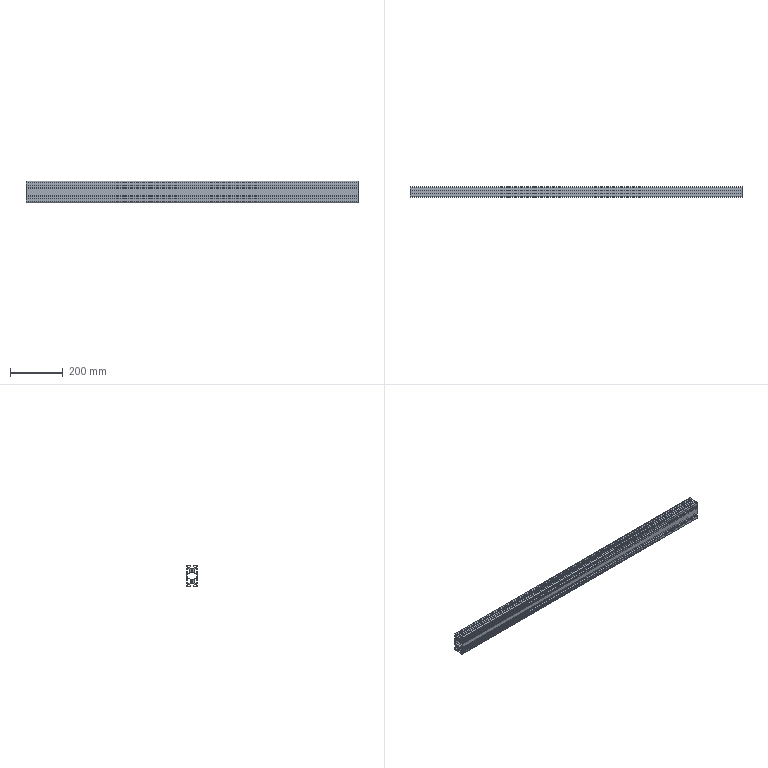Part | 1 solid | 155 faces | box 1260 x 40.002 x 80 mm | volume 1240335 mm3 | plane 142 | cylinder 13 | commonest cylinder face diameters 9 x5 5 x4 6.8 x4